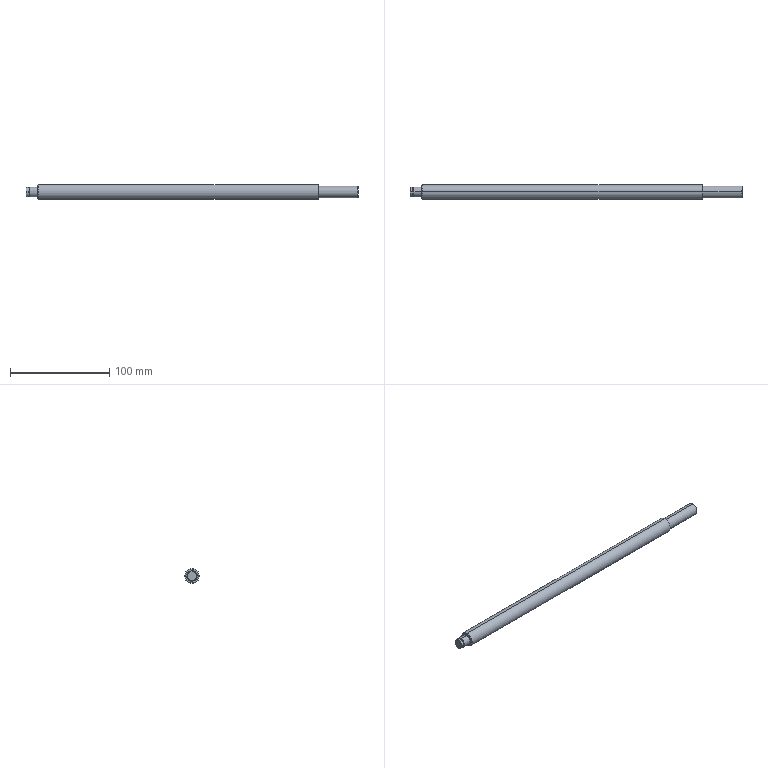Part | SolidWorks | features BaseBody 1 | 1 solid | 26 faces | box 335 x 15 x 15 mm | volume 55455 mm3 | cylinder 10 | cone 6 | plane 6 | spline 4 | commonest cylinder face diameters 10 x4 9.6 x2 12 x2 15 x2
STEP:
#1=CARTESIAN_POINT('',(295.3,0.,-6.));
#2=VERTEX_POINT('',#1);
#3=CARTESIAN_POINT('',(295.3,0.,6.));
#4=VERTEX_POINT('',#3);
#5=CARTESIAN_POINT('',(295.3,0.,0.));
#6=DIRECTION('',(1.,0.,0.));
#7=DIRECTION('',(0.,0.,1.));
#8=AXIS2_PLACEMENT_3D('',#5,#6,#7);
#9=CIRCLE('',#8,6.);
#10=EDGE_CURVE('',#2,#4,#9,.T.);
#11=ORIENTED_EDGE('',*,*,#10,.F.);
#12=CARTESIAN_POINT('',(295.,0.,-6.3));
#13=VERTEX_POINT('',#12);
#14=CARTESIAN_POINT('',(295.3,0.,-6.3));
#15=DIRECTION('',(0.,-1.,0.));
#16=DIRECTION('',(0.,0.,-1.));
#17=AXIS2_PLACEMENT_3D('',#14,#15,#16);
#18=CIRCLE('',#17,0.3);
#19=EDGE_CURVE('',#2,#13,#18,.T.);
#20=ORIENTED_EDGE('',*,*,#19,.T.);
#21=CARTESIAN_POINT('',(295.,0.,6.3));
#22=VERTEX_POINT('',#21);
#23=CARTESIAN_POINT('',(295.,0.,-6.3));
#24=CARTESIAN_POINT('',(295.,12.6,-6.3));
#25=CARTESIAN_POINT('',(295.,12.6,6.3));
#26=CARTESIAN_POINT('',(295.,0.,6.3));
#27=(BOUNDED_CURVE()B_SPLINE_CURVE(3,(#23,#24,#25,#26),.UNSPECIFIED.,.F.,.F.)B_SPLINE_CURVE_WITH_KNOTS((4,4),(0.,1.),.UNSPECIFIED.)CURVE()GEOMETRIC_REPRESENTATION_ITEM()RATIONAL_B_SPLINE_CURVE((1.,0.3333,0.3333,1.))REPRESENTATION_ITEM(''));
#28=EDGE_CURVE('',#13,#22,#27,.T.);
#29=ORIENTED_EDGE('',*,*,#28,.T.);
#30=CARTESIAN_POINT('',(295.3,0.,6.3));
#31=DIRECTION('',(0.,1.,0.));
#32=DIRECTION('',(0.,0.,1.));
#33=AXIS2_PLACEMENT_3D('',#30,#31,#32);
#34=CIRCLE('',#33,0.3);
#35=EDGE_CURVE('',#4,#22,#34,.T.);
#36=ORIENTED_EDGE('',*,*,#35,.F.);
#37=EDGE_LOOP('',(#11,#20,#29,#36));
#38=FACE_OUTER_BOUND('',#37,.T.);
#39=CARTESIAN_POINT('',(295.3,0.,6.));
#40=CARTESIAN_POINT('',(295.3,12.,6.));
#41=CARTESIAN_POINT('',(295.3,12.,-6.));
#42=CARTESIAN_POINT('',(295.3,0.,-6.));
#43=CARTESIAN_POINT('',(295.124,0.,6.));
#44=CARTESIAN_POINT('',(295.124,12.,6.));
#45=CARTESIAN_POINT('',(295.124,12.,-6.));
#46=CARTESIAN_POINT('',(295.124,0.,-6.));
#47=CARTESIAN_POINT('',(295.,0.,6.124));
#48=CARTESIAN_POINT('',(295.,12.249,6.124));
#49=CARTESIAN_POINT('',(295.,12.249,-6.124));
#50=CARTESIAN_POINT('',(295.,0.,-6.124));
#51=CARTESIAN_POINT('',(295.,0.,6.3));
#52=CARTESIAN_POINT('',(295.,12.6,6.3));
#53=CARTESIAN_POINT('',(295.,12.6,-6.3));
#54=CARTESIAN_POINT('',(295.,0.,-6.3));
#55=(BOUNDED_SURFACE()B_SPLINE_SURFACE(3,3,((#39,#40,#41,#42),(#43,#44,#45,#46),(#47,#48,#49,#50),(#51,#52,#53,#54)),.UNSPECIFIED.,.F.,.F.,.T.)B_SPLINE_SURFACE_WITH_KNOTS((4,4),(4,4),(0.,1.),(0.,1.),.UNSPECIFIED.)GEOMETRIC_REPRESENTATION_ITEM()RATIONAL_B_SPLINE_SURFACE(((1.,0.3333,0.3333,1.),(0.8047,0.2682,0.2682,0.8047),(0.8047,0.2682,0.2682,0.8047),(1.,0.3333,0.3333,1.)))REPRESENTATION_ITEM('')SURFACE());
#56=ADVANCED_FACE('',(#38),#55,.F.);
#57=CARTESIAN_POINT('',(12.,0.,5.3));
#58=VERTEX_POINT('',#57);
#59=CARTESIAN_POINT('',(12.,0.,-5.3));
#60=VERTEX_POINT('',#59);
#61=CARTESIAN_POINT('',(12.,0.,5.3));
#62=CARTESIAN_POINT('',(12.,10.6,5.3));
#63=CARTESIAN_POINT('',(12.,10.6,-5.3));
#64=CARTESIAN_POINT('',(12.,0.,-5.3));
#65=(BOUNDED_CURVE()B_SPLINE_CURVE(3,(#61,#62,#63,#64),.UNSPECIFIED.,.F.,.F.)B_SPLINE_CURVE_WITH_KNOTS((4,4),(0.,1.),.UNSPECIFIED.)CURVE()GEOMETRIC_REPRESENTATION_ITEM()RATIONAL_B_SPLINE_CURVE((1.,0.3333,0.3333,1.))REPRESENTATION_ITEM(''));
#66=EDGE_CURVE('',#58,#60,#65,.T.);
#67=ORIENTED_EDGE('',*,*,#66,.T.);
#68=CARTESIAN_POINT('',(11.7,0.,-5.));
#69=VERTEX_POINT('',#68);
#70=CARTESIAN_POINT('',(11.7,0.,-5.3));
#71=DIRECTION('',(0.,-1.,0.));
#72=DIRECTION('',(0.,0.,-1.));
#73=AXIS2_PLACEMENT_3D('',#70,#71,#72);
#74=CIRCLE('',#73,0.3);
#75=EDGE_CURVE('',#60,#69,#74,.T.);
#76=ORIENTED_EDGE('',*,*,#75,.T.);
#77=CARTESIAN_POINT('',(11.7,0.,5.));
#78=VERTEX_POINT('',#77);
#79=CARTESIAN_POINT('',(11.7,0.,0.));
#80=DIRECTION('',(-1.,0.,0.));
#81=DIRECTION('',(0.,0.,1.));
#82=AXIS2_PLACEMENT_3D('',#79,#80,#81);
#83=CIRCLE('',#82,5.);
#84=EDGE_CURVE('',#78,#69,#83,.T.);
#85=ORIENTED_EDGE('',*,*,#84,.F.);
#86=CARTESIAN_POINT('',(11.7,0.,5.3));
#87=DIRECTION('',(0.,1.,0.));
#88=DIRECTION('',(0.,0.,1.));
#89=AXIS2_PLACEMENT_3D('',#86,#87,#88);
#90=CIRCLE('',#89,0.3);
#91=EDGE_CURVE('',#58,#78,#90,.T.);
#92=ORIENTED_EDGE('',*,*,#91,.F.);
#93=EDGE_LOOP('',(#67,#76,#85,#92));
#94=FACE_OUTER_BOUND('',#93,.T.);
#95=CARTESIAN_POINT('',(12.,0.,5.3));
#96=CARTESIAN_POINT('',(12.,10.6,5.3));
#97=CARTESIAN_POINT('',(12.,10.6,-5.3));
#98=CARTESIAN_POINT('',(12.,0.,-5.3));
#99=CARTESIAN_POINT('',(12.,0.,5.124));
#100=CARTESIAN_POINT('',(12.,10.249,5.124));
#101=CARTESIAN_POINT('',(12.,10.249,-5.124));
#102=CARTESIAN_POINT('',(12.,0.,-5.124));
#103=CARTESIAN_POINT('',(11.876,0.,5.));
#104=CARTESIAN_POINT('',(11.876,10.,5.));
#105=CARTESIAN_POINT('',(11.876,10.,-5.));
#106=CARTESIAN_POINT('',(11.876,0.,-5.));
#107=CARTESIAN_POINT('',(11.7,0.,5.));
#108=CARTESIAN_POINT('',(11.7,10.,5.));
#109=CARTESIAN_POINT('',(11.7,10.,-5.));
#110=CARTESIAN_POINT('',(11.7,0.,-5.));
#111=(BOUNDED_SURFACE()B_SPLINE_SURFACE(3,3,((#95,#96,#97,#98),(#99,#100,#101,#102),(#103,#104,#105,#106),(#107,#108,#109,#110)),.UNSPECIFIED.,.F.,.F.,.T.)B_SPLINE_SURFACE_WITH_KNOTS((4,4),(4,4),(0.,1.),(0.,1.),.UNSPECIFIED.)GEOMETRIC_REPRESENTATION_ITEM()RATIONAL_B_SPLINE_SURFACE(((1.,0.3333,0.3333,1.),(0.8047,0.2682,0.2682,0.8047),(0.8047,0.2682,0.2682,0.8047),(1.,0.3333,0.3333,1.)))REPRESENTATION_ITEM('')SURFACE());
#112=ADVANCED_FACE('',(#94),#111,.F.);
#113=CARTESIAN_POINT('',(295.,0.,7.5));
#114=VERTEX_POINT('',#113);
#115=CARTESIAN_POINT('',(295.,0.,-7.5));
#116=VERTEX_POINT('',#115);
#117=CARTESIAN_POINT('',(295.,0.,0.));
#118=DIRECTION('',(-1.,0.,0.));
#119=DIRECTION('',(0.,0.,1.));
#120=AXIS2_PLACEMENT_3D('',#117,#118,#119);
#121=CIRCLE('',#120,7.5);
#122=EDGE_CURVE('',#114,#116,#121,.T.);
#123=ORIENTED_EDGE('',*,*,#122,.T.);
#124=CARTESIAN_POINT('',(12.5,0.,-7.5));
#125=VERTEX_POINT('',#124);
#126=CARTESIAN_POINT('',(350.,0.,-7.5));
#127=DIRECTION('',(-1.,0.,0.));
#128=VECTOR('',#127,1000.);
#129=LINE('',#126,#128);
#130=EDGE_CURVE('',#116,#125,#129,.T.);
#131=ORIENTED_EDGE('',*,*,#130,.T.);
#132=CARTESIAN_POINT('',(12.5,0.,7.5));
#133=VERTEX_POINT('',#132);
#134=CARTESIAN_POINT('',(12.5,0.,0.));
#135=DIRECTION('',(1.,0.,0.));
#136=DIRECTION('',(0.,0.,1.));
#137=AXIS2_PLACEMENT_3D('',#134,#135,#136);
#138=CIRCLE('',#137,7.5);
#139=EDGE_CURVE('',#125,#133,#138,.T.);
#140=ORIENTED_EDGE('',*,*,#139,.T.);
#141=CARTESIAN_POINT('',(350.,0.,7.5));
#142=DIRECTION('',(-1.,0.,0.));
#143=VECTOR('',#142,1000.);
#144=LINE('',#141,#143);
#145=EDGE_CURVE('',#114,#133,#144,.T.);
#146=ORIENTED_EDGE('',*,*,#145,.F.);
#147=EDGE_LOOP('',(#123,#131,#140,#146));
#148=FACE_OUTER_BOUND('',#147,.T.);
#149=CARTESIAN_POINT('',(350.,0.,0.));
#150=DIRECTION('',(-1.,0.,0.));
#151=DIRECTION('',(0.,0.,1.));
#152=AXIS2_PLACEMENT_3D('',#149,#150,#151);
#153=CYLINDRICAL_SURFACE('',#152,7.5);
#154=ADVANCED_FACE('',(#148),#153,.T.);
#155=CARTESIAN_POINT('',(12.,0.,-7.));
#156=VERTEX_POINT('',#155);
#157=CARTESIAN_POINT('',(12.,0.,7.));
#158=VERTEX_POINT('',#157);
#159=CARTESIAN_POINT('',(12.,0.,0.));
#160=DIRECTION('',(1.,0.,0.));
#161=DIRECTION('',(0.,0.,-1.));
#162=AXIS2_PLACEMENT_3D('',#159,#160,#161);
#163=CIRCLE('',#162,7.);
#164=EDGE_CURVE('',#156,#158,#163,.T.);
#165=ORIENTED_EDGE('',*,*,#164,.T.);
#166=CARTESIAN_POINT('',(12.5,0.,7.5));
#167=DIRECTION('',(0.7071,0.,0.7071));
#168=VECTOR('',#167,1000.);
#169=LINE('',#166,#168);
#170=EDGE_CURVE('',#158,#133,#169,.T.);
#171=ORIENTED_EDGE('',*,*,#170,.T.);
#172=ORIENTED_EDGE('',*,*,#139,.F.);
#173=CARTESIAN_POINT('',(12.5,0.,-7.5));
#174=DIRECTION('',(0.7071,0.,-0.7071));
#175=VECTOR('',#174,1000.);
#176=LINE('',#173,#175);
#177=EDGE_CURVE('',#156,#125,#176,.T.);
#178=ORIENTED_EDGE('',*,*,#177,.F.);
#179=EDGE_LOOP('',(#165,#171,#172,#178));
#180=FACE_OUTER_BOUND('',#179,.T.);
#181=CARTESIAN_POINT('',(12.5,0.,0.));
#182=DIRECTION('',(1.,0.,0.));
#183=DIRECTION('',(0.,0.,-1.));
#184=AXIS2_PLACEMENT_3D('',#181,#182,#183);
#185=CONICAL_SURFACE('',#184,7.5,0.7854);
#186=ADVANCED_FACE('',(#180),#185,.T.);
#187=CARTESIAN_POINT('',(334.5,0.,6.));
#188=VERTEX_POINT('',#187);
#189=CARTESIAN_POINT('',(334.5,0.,-6.));
#190=VERTEX_POINT('',#189);
#191=CARTESIAN_POINT('',(334.5,0.,0.));
#192=DIRECTION('',(-1.,0.,0.));
#193=DIRECTION('',(0.,0.,1.));
#194=AXIS2_PLACEMENT_3D('',#191,#192,#193);
#195=CIRCLE('',#194,6.);
#196=EDGE_CURVE('',#188,#190,#195,.T.);
#197=ORIENTED_EDGE('',*,*,#196,.T.);
#198=CARTESIAN_POINT('',(350.,0.,-6.));
#199=DIRECTION('',(-1.,0.,0.));
#200=VECTOR('',#199,1000.);
#201=LINE('',#198,#200);
#202=EDGE_CURVE('',#190,#2,#201,.T.);
#203=ORIENTED_EDGE('',*,*,#202,.T.);
#204=ORIENTED_EDGE('',*,*,#10,.T.);
#205=CARTESIAN_POINT('',(350.,0.,6.));
#206=DIRECTION('',(-1.,0.,0.));
#207=VECTOR('',#206,1000.);
#208=LINE('',#205,#207);
#209=EDGE_CURVE('',#188,#4,#208,.T.);
#210=ORIENTED_EDGE('',*,*,#209,.F.);
#211=EDGE_LOOP('',(#197,#203,#204,#210));
#212=FACE_OUTER_BOUND('',#211,.T.);
#213=CARTESIAN_POINT('',(350.,0.,0.));
#214=DIRECTION('',(-1.,0.,0.));
#215=DIRECTION('',(0.,0.,1.));
#216=AXIS2_PLACEMENT_3D('',#213,#214,#215);
#217=CYLINDRICAL_SURFACE('',#216,6.);
#218=ADVANCED_FACE('',(#212),#217,.T.);
#219=ORIENTED_EDGE('',*,*,#84,.T.);
#220=CARTESIAN_POINT('',(4.,0.,-5.));
#221=VERTEX_POINT('',#220);
#222=CARTESIAN_POINT('',(350.,0.,-5.));
#223=DIRECTION('',(-1.,0.,0.));
#224=VECTOR('',#223,1000.);
#225=LINE('',#222,#224);
#226=EDGE_CURVE('',#69,#221,#225,.T.);
#227=ORIENTED_EDGE('',*,*,#226,.T.);
#228=CARTESIAN_POINT('',(4.,0.,5.));
#229=VERTEX_POINT('',#228);
#230=CARTESIAN_POINT('',(4.,0.,0.));
#231=DIRECTION('',(1.,0.,0.));
#232=DIRECTION('',(0.,0.,1.));
#233=AXIS2_PLACEMENT_3D('',#230,#231,#232);
#234=CIRCLE('',#233,5.);
#235=EDGE_CURVE('',#221,#229,#234,.T.);
#236=ORIENTED_EDGE('',*,*,#235,.T.);
#237=CARTESIAN_POINT('',(350.,0.,5.));
#238=DIRECTION('',(-1.,0.,0.));
#239=VECTOR('',#238,1000.);
#240=LINE('',#237,#239);
#241=EDGE_CURVE('',#78,#229,#240,.T.);
#242=ORIENTED_EDGE('',*,*,#241,.F.);
#243=EDGE_LOOP('',(#219,#227,#236,#242));
#244=FACE_OUTER_BOUND('',#243,.T.);
#245=CARTESIAN_POINT('',(350.,0.,0.));
#246=DIRECTION('',(-1.,0.,0.));
#247=DIRECTION('',(0.,0.,1.));
#248=AXIS2_PLACEMENT_3D('',#245,#246,#247);
#249=CYLINDRICAL_SURFACE('',#248,5.);
#250=ADVANCED_FACE('',(#244),#249,.T.);
#251=CARTESIAN_POINT('',(335.,0.,5.5));
#252=VERTEX_POINT('',#251);
#253=CARTESIAN_POINT('',(335.,0.,-5.5));
#254=VERTEX_POINT('',#253);
#255=CARTESIAN_POINT('',(335.,0.,0.));
#256=DIRECTION('',(-1.,0.,0.));
#257=DIRECTION('',(0.,0.,1.));
#258=AXIS2_PLACEMENT_3D('',#255,#256,#257);
#259=CIRCLE('',#258,5.5);
#260=EDGE_CURVE('',#252,#254,#259,.T.);
#261=ORIENTED_EDGE('',*,*,#260,.T.);
#262=CARTESIAN_POINT('',(334.5,0.,-6.));
#263=DIRECTION('',(-0.7071,0.,-0.7071));
#264=VECTOR('',#263,1000.);
#265=LINE('',#262,#264);
#266=EDGE_CURVE('',#254,#190,#265,.T.);
#267=ORIENTED_EDGE('',*,*,#266,.T.);
#268=ORIENTED_EDGE('',*,*,#196,.F.);
#269=CARTESIAN_POINT('',(334.5,0.,6.));
#270=DIRECTION('',(-0.7071,0.,0.7071));
#271=VECTOR('',#270,1000.);
#272=LINE('',#269,#271);
#273=EDGE_CURVE('',#252,#188,#272,.T.);
#274=ORIENTED_EDGE('',*,*,#273,.F.);
#275=EDGE_LOOP('',(#261,#267,#268,#274));
#276=FACE_OUTER_BOUND('',#275,.T.);
#277=CARTESIAN_POINT('',(334.5,0.,0.));
#278=DIRECTION('',(-1.,0.,0.));
#279=DIRECTION('',(0.,0.,1.));
#280=AXIS2_PLACEMENT_3D('',#277,#278,#279);
#281=CONICAL_SURFACE('',#280,6.,0.7854);
#282=ADVANCED_FACE('',(#276),#281,.T.);
#283=CARTESIAN_POINT('',(4.,0.,4.8));
#284=VERTEX_POINT('',#283);
#285=CARTESIAN_POINT('',(4.,0.,-4.8));
#286=VERTEX_POINT('',#285);
#287=CARTESIAN_POINT('',(4.,0.,0.));
#288=DIRECTION('',(-1.,0.,0.));
#289=DIRECTION('',(0.,0.,1.));
#290=AXIS2_PLACEMENT_3D('',#287,#288,#289);
#291=CIRCLE('',#290,4.8);
#292=EDGE_CURVE('',#284,#286,#291,.T.);
#293=ORIENTED_EDGE('',*,*,#292,.T.);
#294=CARTESIAN_POINT('',(2.85,0.,-4.8));
#295=VERTEX_POINT('',#294);
#296=CARTESIAN_POINT('',(350.,0.,-4.8));
#297=DIRECTION('',(-1.,0.,0.));
#298=VECTOR('',#297,1000.);
#299=LINE('',#296,#298);
#300=EDGE_CURVE('',#286,#295,#299,.T.);
#301=ORIENTED_EDGE('',*,*,#300,.T.);
#302=CARTESIAN_POINT('',(2.85,0.,4.8));
#303=VERTEX_POINT('',#302);
#304=CARTESIAN_POINT('',(2.85,0.,0.));
#305=DIRECTION('',(1.,0.,0.));
#306=DIRECTION('',(0.,0.,1.));
#307=AXIS2_PLACEMENT_3D('',#304,#305,#306);
#308=CIRCLE('',#307,4.8);
#309=EDGE_CURVE('',#295,#303,#308,.T.);
#310=ORIENTED_EDGE('',*,*,#309,.T.);
#311=CARTESIAN_POINT('',(350.,0.,4.8));
#312=DIRECTION('',(-1.,0.,0.));
#313=VECTOR('',#312,1000.);
#314=LINE('',#311,#313);
#315=EDGE_CURVE('',#284,#303,#314,.T.);
#316=ORIENTED_EDGE('',*,*,#315,.F.);
#317=EDGE_LOOP('',(#293,#301,#310,#316));
#318=FACE_OUTER_BOUND('',#317,.T.);
#319=CARTESIAN_POINT('',(350.,0.,0.));
#320=DIRECTION('',(-1.,0.,0.));
#321=DIRECTION('',(0.,0.,1.));
#322=AXIS2_PLACEMENT_3D('',#319,#320,#321);
#323=CYLINDRICAL_SURFACE('',#322,4.8);
#324=ADVANCED_FACE('',(#318),#323,.T.);
#325=CARTESIAN_POINT('',(2.85,0.,5.));
#326=VERTEX_POINT('',#325);
#327=CARTESIAN_POINT('',(2.85,0.,-5.));
#328=VERTEX_POINT('',#327);
#329=CARTESIAN_POINT('',(2.85,0.,0.));
#330=DIRECTION('',(-1.,0.,0.));
#331=DIRECTION('',(0.,0.,1.));
#332=AXIS2_PLACEMENT_3D('',#329,#330,#331);
#333=CIRCLE('',#332,5.);
#334=EDGE_CURVE('',#326,#328,#333,.T.);
#335=ORIENTED_EDGE('',*,*,#334,.T.);
#336=CARTESIAN_POINT('',(0.5,0.,-5.));
#337=VERTEX_POINT('',#336);
#338=CARTESIAN_POINT('',(350.,0.,-5.));
#339=DIRECTION('',(-1.,0.,0.));
#340=VECTOR('',#339,1000.);
#341=LINE('',#338,#340);
#342=EDGE_CURVE('',#328,#337,#341,.T.);
#343=ORIENTED_EDGE('',*,*,#342,.T.);
#344=CARTESIAN_POINT('',(0.5,0.,5.));
#345=VERTEX_POINT('',#344);
#346=CARTESIAN_POINT('',(0.5,0.,0.));
#347=DIRECTION('',(1.,0.,0.));
#348=DIRECTION('',(0.,0.,1.));
#349=AXIS2_PLACEMENT_3D('',#346,#347,#348);
#350=CIRCLE('',#349,5.);
#351=EDGE_CURVE('',#337,#345,#350,.T.);
#352=ORIENTED_EDGE('',*,*,#351,.T.);
#353=CARTESIAN_POINT('',(350.,0.,5.));
#354=DIRECTION('',(-1.,0.,0.));
#355=VECTOR('',#354,1000.);
#356=LINE('',#353,#355);
#357=EDGE_CURVE('',#326,#345,#356,.T.);
#358=ORIENTED_EDGE('',*,*,#357,.F.);
#359=EDGE_LOOP('',(#335,#343,#352,#358));
#360=FACE_OUTER_BOUND('',#359,.T.);
#361=CARTESIAN_POINT('',(350.,0.,0.));
#362=DIRECTION('',(-1.,0.,0.));
#363=DIRECTION('',(0.,0.,1.));
#364=AXIS2_PLACEMENT_3D('',#361,#362,#363);
#365=CYLINDRICAL_SURFACE('',#364,5.);
#366=ADVANCED_FACE('',(#360),#365,.T.);
#367=CARTESIAN_POINT('',(0.,0.,-4.5));
#368=VERTEX_POINT('',#367);
#369=CARTESIAN_POINT('',(0.,0.,4.5));
#370=VERTEX_POINT('',#369);
#371=CARTESIAN_POINT('',(0.,0.,0.));
#372=DIRECTION('',(1.,0.,0.));
#373=DIRECTION('',(0.,0.,-1.));
#374=AXIS2_PLACEMENT_3D('',#371,#372,#373);
#375=CIRCLE('',#374,4.5);
#376=EDGE_CURVE('',#368,#370,#375,.T.);
#377=ORIENTED_EDGE('',*,*,#376,.T.);
#378=CARTESIAN_POINT('',(0.5,0.,5.));
#379=DIRECTION('',(0.7071,0.,0.7071));
#380=VECTOR('',#379,1000.);
#381=LINE('',#378,#380);
#382=EDGE_CURVE('',#370,#345,#381,.T.);
#383=ORIENTED_EDGE('',*,*,#382,.T.);
#384=ORIENTED_EDGE('',*,*,#351,.F.);
#385=CARTESIAN_POINT('',(0.5,0.,-5.));
#386=DIRECTION('',(0.7071,0.,-0.7071));
#387=VECTOR('',#386,1000.);
#388=LINE('',#385,#387);
#389=EDGE_CURVE('',#368,#337,#388,.T.);
#390=ORIENTED_EDGE('',*,*,#389,.F.);
#391=EDGE_LOOP('',(#377,#383,#384,#390));
#392=FACE_OUTER_BOUND('',#391,.T.);
#393=CARTESIAN_POINT('',(0.5,0.,0.));
#394=DIRECTION('',(1.,0.,0.));
#395=DIRECTION('',(0.,0.,-1.));
#396=AXIS2_PLACEMENT_3D('',#393,#394,#395);
#397=CONICAL_SURFACE('',#396,5.,0.7854);
#398=ADVANCED_FACE('',(#392),#397,.T.);
#399=ORIENTED_EDGE('',*,*,#130,.F.);
#400=CARTESIAN_POINT('',(295.,0.,0.));
#401=DIRECTION('',(-1.,0.,0.));
#402=DIRECTION('',(0.,0.,1.));
#403=AXIS2_PLACEMENT_3D('',#400,#401,#402);
#404=CIRCLE('',#403,7.5);
#405=EDGE_CURVE('',#116,#114,#404,.T.);
#406=ORIENTED_EDGE('',*,*,#405,.T.);
#407=ORIENTED_EDGE('',*,*,#145,.T.);
#408=CARTESIAN_POINT('',(12.5,0.,0.));
#409=DIRECTION('',(1.,0.,0.));
#410=DIRECTION('',(0.,0.,1.));
#411=AXIS2_PLACEMENT_3D('',#408,#409,#410);
#412=CIRCLE('',#411,7.5);
#413=EDGE_CURVE('',#133,#125,#412,.T.);
#414=ORIENTED_EDGE('',*,*,#413,.T.);
#415=EDGE_LOOP('',(#399,#406,#407,#414));
#416=FACE_OUTER_BOUND('',#415,.T.);
#417=CARTESIAN_POINT('',(350.,0.,0.));
#418=DIRECTION('',(-1.,0.,0.));
#419=DIRECTION('',(0.,0.,1.));
#420=AXIS2_PLACEMENT_3D('',#417,#418,#419);
#421=CYLINDRICAL_SURFACE('',#420,7.5);
#422=ADVANCED_FACE('',(#416),#421,.T.);
#423=ORIENTED_EDGE('',*,*,#170,.F.);
#424=CARTESIAN_POINT('',(12.,0.,0.));
#425=DIRECTION('',(1.,0.,0.));
#426=DIRECTION('',(0.,0.,-1.));
#427=AXIS2_PLACEMENT_3D('',#424,#425,#426);
#428=CIRCLE('',#427,7.);
#429=EDGE_CURVE('',#158,#156,#428,.T.);
#430=ORIENTED_EDGE('',*,*,#429,.T.);
#431=ORIENTED_EDGE('',*,*,#177,.T.);
#432=ORIENTED_EDGE('',*,*,#413,.F.);
#433=EDGE_LOOP('',(#423,#430,#431,#432));
#434=FACE_OUTER_BOUND('',#433,.T.);
#435=CARTESIAN_POINT('',(12.5,0.,0.));
#436=DIRECTION('',(1.,0.,0.));
#437=DIRECTION('',(0.,0.,-1.));
#438=AXIS2_PLACEMENT_3D('',#435,#436,#437);
#439=CONICAL_SURFACE('',#438,7.5,0.7854);
#440=ADVANCED_FACE('',(#434),#439,.T.);
#441=CARTESIAN_POINT('',(295.,0.,6.3));
#442=CARTESIAN_POINT('',(295.,-12.6,6.3));
#443=CARTESIAN_POINT('',(295.,-12.6,-6.3));
#444=CARTESIAN_POINT('',(295.,0.,-6.3));
#445=(BOUNDED_CURVE()B_SPLINE_CURVE(3,(#441,#442,#443,#444),.UNSPECIFIED.,.F.,.F.)B_SPLINE_CURVE_WITH_KNOTS((4,4),(0.,1.),.UNSPECIFIED.)CURVE()GEOMETRIC_REPRESENTATION_ITEM()RATIONAL_B_SPLINE_CURVE((1.,0.3333,0.3333,1.))REPRESENTATION_ITEM(''));
#446=EDGE_CURVE('',#22,#13,#445,.T.);
#447=ORIENTED_EDGE('',*,*,#446,.F.);
#448=ORIENTED_EDGE('',*,*,#28,.F.);
#449=EDGE_LOOP('',(#447,#448));
#450=FACE_BOUND('',#449,.T.);
#451=ORIENTED_EDGE('',*,*,#122,.F.);
#452=ORIENTED_EDGE('',*,*,#405,.F.);
#453=EDGE_LOOP('',(#451,#452));
#454=FACE_OUTER_BOUND('',#453,.T.);
#455=CARTESIAN_POINT('',(295.,7.5,0.));
#456=DIRECTION('',(-1.,0.,0.));
#457=DIRECTION('',(0.,0.,1.));
#458=AXIS2_PLACEMENT_3D('',#455,#456,#457);
#459=PLANE('',#458);
#460=ADVANCED_FACE('',(#450,#454),#459,.F.);
#461=ORIENTED_EDGE('',*,*,#164,.F.);
#462=ORIENTED_EDGE('',*,*,#429,.F.);
#463=EDGE_LOOP('',(#461,#462));
#464=FACE_OUTER_BOUND('',#463,.T.);
#465=CARTESIAN_POINT('',(12.,0.,-5.3));
#466=CARTESIAN_POINT('',(12.,-10.6,-5.3));
#467=CARTESIAN_POINT('',(12.,-10.6,5.3));
#468=CARTESIAN_POINT('',(12.,0.,5.3));
#469=(BOUNDED_CURVE()B_SPLINE_CURVE(3,(#465,#466,#467,#468),.UNSPECIFIED.,.F.,.F.)B_SPLINE_CURVE_WITH_KNOTS((4,4),(0.,1.),.UNSPECIFIED.)CURVE()GEOMETRIC_REPRESENTATION_ITEM()RATIONAL_B_SPLINE_CURVE((1.,0.3333,0.3333,1.))REPRESENTATION_ITEM(''));
#470=EDGE_CURVE('',#60,#58,#469,.T.);
#471=ORIENTED_EDGE('',*,*,#470,.F.);
#472=ORIENTED_EDGE('',*,*,#66,.F.);
#473=EDGE_LOOP('',(#471,#472));
#474=FACE_BOUND('',#473,.T.);
#475=CARTESIAN_POINT('',(12.,5.3,0.));
#476=DIRECTION('',(1.,0.,0.));
#477=DIRECTION('',(0.,0.,-1.));
#478=AXIS2_PLACEMENT_3D('',#475,#476,#477);
#479=PLANE('',#478);
#480=ADVANCED_FACE('',(#464,#474),#479,.F.);
#481=ORIENTED_EDGE('',*,*,#19,.F.);
#482=CARTESIAN_POINT('',(295.3,0.,0.));
#483=DIRECTION('',(1.,0.,0.));
#484=DIRECTION('',(0.,0.,1.));
#485=AXIS2_PLACEMENT_3D('',#482,#483,#484);
#486=CIRCLE('',#485,6.);
#487=EDGE_CURVE('',#4,#2,#486,.T.);
#488=ORIENTED_EDGE('',*,*,#487,.F.);
#489=ORIENTED_EDGE('',*,*,#35,.T.);
#490=ORIENTED_EDGE('',*,*,#446,.T.);
#491=EDGE_LOOP('',(#481,#488,#489,#490));
#492=FACE_OUTER_BOUND('',#491,.T.);
#493=CARTESIAN_POINT('',(295.3,0.,-6.));
#494=CARTESIAN_POINT('',(295.3,-12.,-6.));
#495=CARTESIAN_POINT('',(295.3,-12.,6.));
#496=CARTESIAN_POINT('',(295.3,0.,6.));
#497=CARTESIAN_POINT('',(295.124,0.,-6.));
#498=CARTESIAN_POINT('',(295.124,-12.,-6.));
#499=CARTESIAN_POINT('',(295.124,-12.,6.));
#500=CARTESIAN_POINT('',(295.124,0.,6.));
#501=CARTESIAN_POINT('',(295.,0.,-6.124));
#502=CARTESIAN_POINT('',(295.,-12.249,-6.124));
#503=CARTESIAN_POINT('',(295.,-12.249,6.124));
#504=CARTESIAN_POINT('',(295.,0.,6.124));
#505=CARTESIAN_POINT('',(295.,0.,-6.3));
#506=CARTESIAN_POINT('',(295.,-12.6,-6.3));
#507=CARTESIAN_POINT('',(295.,-12.6,6.3));
#508=CARTESIAN_POINT('',(295.,0.,6.3));
#509=(BOUNDED_SURFACE()B_SPLINE_SURFACE(3,3,((#493,#494,#495,#496),(#497,#498,#499,#500),(#501,#502,#503,#504),(#505,#506,#507,#508)),.UNSPECIFIED.,.F.,.F.,.T.)B_SPLINE_SURFACE_WITH_KNOTS((4,4),(4,4),(0.,1.),(0.,1.),.UNSPECIFIED.)GEOMETRIC_REPRESENTATION_ITEM()RATIONAL_B_SPLINE_SURFACE(((1.,0.3333,0.3333,1.),(0.8047,0.2682,0.2682,0.8047),(0.8047,0.2682,0.2682,0.8047),(1.,0.3333,0.3333,1.)))REPRESENTATION_ITEM('')SURFACE());
#510=ADVANCED_FACE('',(#492),#509,.F.);
#511=ORIENTED_EDGE('',*,*,#75,.F.);
#512=ORIENTED_EDGE('',*,*,#470,.T.);
#513=ORIENTED_EDGE('',*,*,#91,.T.);
#514=CARTESIAN_POINT('',(11.7,0.,0.));
#515=DIRECTION('',(-1.,0.,0.));
#516=DIRECTION('',(0.,0.,1.));
#517=AXIS2_PLACEMENT_3D('',#514,#515,#516);
#518=CIRCLE('',#517,5.);
#519=EDGE_CURVE('',#69,#78,#518,.T.);
#520=ORIENTED_EDGE('',*,*,#519,.F.);
#521=EDGE_LOOP('',(#511,#512,#513,#520));
#522=FACE_OUTER_BOUND('',#521,.T.);
#523=CARTESIAN_POINT('',(12.,0.,-5.3));
#524=CARTESIAN_POINT('',(12.,-10.6,-5.3));
#525=CARTESIAN_POINT('',(12.,-10.6,5.3));
#526=CARTESIAN_POINT('',(12.,0.,5.3));
#527=CARTESIAN_POINT('',(12.,0.,-5.124));
#528=CARTESIAN_POINT('',(12.,-10.249,-5.124));
#529=CARTESIAN_POINT('',(12.,-10.249,5.124));
#530=CARTESIAN_POINT('',(12.,0.,5.124));
#531=CARTESIAN_POINT('',(11.876,0.,-5.));
#532=CARTESIAN_POINT('',(11.876,-10.,-5.));
#533=CARTESIAN_POINT('',(11.876,-10.,5.));
#534=CARTESIAN_POINT('',(11.876,0.,5.));
#535=CARTESIAN_POINT('',(11.7,0.,-5.));
#536=CARTESIAN_POINT('',(11.7,-10.,-5.));
#537=CARTESIAN_POINT('',(11.7,-10.,5.));
#538=CARTESIAN_POINT('',(11.7,0.,5.));
#539=(BOUNDED_SURFACE()B_SPLINE_SURFACE(3,3,((#523,#524,#525,#526),(#527,#528,#529,#530),(#531,#532,#533,#534),(#535,#536,#537,#538)),.UNSPECIFIED.,.F.,.F.,.F.)B_SPLINE_SURFACE_WITH_KNOTS((4,4),(4,4),(0.,1.),(0.,1.),.UNSPECIFIED.)GEOMETRIC_REPRESENTATION_ITEM()RATIONAL_B_SPLINE_SURFACE(((1.,0.3333,0.3333,1.),(0.8047,0.2682,0.2682,0.8047),(0.8047,0.2682,0.2682,0.8047),(1.,0.3333,0.3333,1.)))REPRESENTATION_ITEM('')SURFACE());
#540=ADVANCED_FACE('',(#522),#539,.F.);
#541=ORIENTED_EDGE('',*,*,#202,.F.);
#542=CARTESIAN_POINT('',(334.5,0.,0.));
#543=DIRECTION('',(-1.,0.,0.));
#544=DIRECTION('',(0.,0.,1.));
#545=AXIS2_PLACEMENT_3D('',#542,#543,#544);
#546=CIRCLE('',#545,6.);
#547=EDGE_CURVE('',#190,#188,#546,.T.);
#548=ORIENTED_EDGE('',*,*,#547,.T.);
#549=ORIENTED_EDGE('',*,*,#209,.T.);
#550=ORIENTED_EDGE('',*,*,#487,.T.);
#551=EDGE_LOOP('',(#541,#548,#549,#550));
#552=FACE_OUTER_BOUND('',#551,.T.);
#553=CARTESIAN_POINT('',(350.,0.,0.));
#554=DIRECTION('',(-1.,0.,0.));
#555=DIRECTION('',(0.,0.,1.));
#556=AXIS2_PLACEMENT_3D('',#553,#554,#555);
#557=CYLINDRICAL_SURFACE('',#556,6.);
#558=ADVANCED_FACE('',(#552),#557,.T.);
#559=ORIENTED_EDGE('',*,*,#226,.F.);
#560=ORIENTED_EDGE('',*,*,#519,.T.);
#561=ORIENTED_EDGE('',*,*,#241,.T.);
#562=CARTESIAN_POINT('',(4.,0.,0.));
#563=DIRECTION('',(1.,0.,0.));
#564=DIRECTION('',(0.,0.,1.));
#565=AXIS2_PLACEMENT_3D('',#562,#563,#564);
#566=CIRCLE('',#565,5.);
#567=EDGE_CURVE('',#229,#221,#566,.T.);
#568=ORIENTED_EDGE('',*,*,#567,.T.);
#569=EDGE_LOOP('',(#559,#560,#561,#568));
#570=FACE_OUTER_BOUND('',#569,.T.);
#571=CARTESIAN_POINT('',(350.,0.,0.));
#572=DIRECTION('',(-1.,0.,0.));
#573=DIRECTION('',(0.,0.,1.));
#574=AXIS2_PLACEMENT_3D('',#571,#572,#573);
#575=CYLINDRICAL_SURFACE('',#574,5.);
#576=ADVANCED_FACE('',(#570),#575,.T.);
#577=ORIENTED_EDGE('',*,*,#266,.F.);
#578=CARTESIAN_POINT('',(335.,0.,0.));
#579=DIRECTION('',(-1.,0.,0.));
#580=DIRECTION('',(0.,0.,1.));
#581=AXIS2_PLACEMENT_3D('',#578,#579,#580);
#582=CIRCLE('',#581,5.5);
#583=EDGE_CURVE('',#254,#252,#582,.T.);
#584=ORIENTED_EDGE('',*,*,#583,.T.);
#585=ORIENTED_EDGE('',*,*,#273,.T.);
#586=ORIENTED_EDGE('',*,*,#547,.F.);
#587=EDGE_LOOP('',(#577,#584,#585,#586));
#588=FACE_OUTER_BOUND('',#587,.T.);
#589=CARTESIAN_POINT('',(334.5,0.,0.));
#590=DIRECTION('',(-1.,0.,0.));
#591=DIRECTION('',(0.,0.,1.));
#592=AXIS2_PLACEMENT_3D('',#589,#590,#591);
#593=CONICAL_SURFACE('',#592,6.,0.7854);
#594=ADVANCED_FACE('',(#588),#593,.T.);
#595=ORIENTED_EDGE('',*,*,#567,.F.);
#596=ORIENTED_EDGE('',*,*,#235,.F.);
#597=EDGE_LOOP('',(#595,#596));
#598=FACE_OUTER_BOUND('',#597,.T.);
#599=ORIENTED_EDGE('',*,*,#292,.F.);
#600=CARTESIAN_POINT('',(4.,0.,0.));
#601=DIRECTION('',(-1.,0.,0.));
#602=DIRECTION('',(0.,0.,1.));
#603=AXIS2_PLACEMENT_3D('',#600,#601,#602);
#604=CIRCLE('',#603,4.8);
#605=EDGE_CURVE('',#286,#284,#604,.T.);
#606=ORIENTED_EDGE('',*,*,#605,.F.);
#607=EDGE_LOOP('',(#599,#606));
#608=FACE_BOUND('',#607,.T.);
#609=CARTESIAN_POINT('',(4.,4.8,0.));
#610=DIRECTION('',(1.,0.,0.));
#611=DIRECTION('',(0.,0.,-1.));
#612=AXIS2_PLACEMENT_3D('',#609,#610,#611);
#613=PLANE('',#612);
#614=ADVANCED_FACE('',(#598,#608),#613,.F.);
#615=ORIENTED_EDGE('',*,*,#260,.F.);
#616=ORIENTED_EDGE('',*,*,#583,.F.);
#617=EDGE_LOOP('',(#615,#616));
#618=FACE_OUTER_BOUND('',#617,.T.);
#619=CARTESIAN_POINT('',(335.,5.5,0.));
#620=DIRECTION('',(-1.,0.,0.));
#621=DIRECTION('',(0.,0.,1.));
#622=AXIS2_PLACEMENT_3D('',#619,#620,#621);
#623=PLANE('',#622);
#624=ADVANCED_FACE('',(#618),#623,.F.);
#625=ORIENTED_EDGE('',*,*,#300,.F.);
#626=ORIENTED_EDGE('',*,*,#605,.T.);
#627=ORIENTED_EDGE('',*,*,#315,.T.);
#628=CARTESIAN_POINT('',(2.85,0.,0.));
#629=DIRECTION('',(1.,0.,0.));
#630=DIRECTION('',(0.,0.,1.));
#631=AXIS2_PLACEMENT_3D('',#628,#629,#630);
#632=CIRCLE('',#631,4.8);
#633=EDGE_CURVE('',#303,#295,#632,.T.);
#634=ORIENTED_EDGE('',*,*,#633,.T.);
#635=EDGE_LOOP('',(#625,#626,#627,#634));
#636=FACE_OUTER_BOUND('',#635,.T.);
#637=CARTESIAN_POINT('',(350.,0.,0.));
#638=DIRECTION('',(-1.,0.,0.));
#639=DIRECTION('',(0.,0.,1.));
#640=AXIS2_PLACEMENT_3D('',#637,#638,#639);
#641=CYLINDRICAL_SURFACE('',#640,4.8);
#642=ADVANCED_FACE('',(#636),#641,.T.);
#643=ORIENTED_EDGE('',*,*,#633,.F.);
#644=ORIENTED_EDGE('',*,*,#309,.F.);
#645=EDGE_LOOP('',(#643,#644));
#646=FACE_BOUND('',#645,.T.);
#647=ORIENTED_EDGE('',*,*,#334,.F.);
#648=CARTESIAN_POINT('',(2.85,0.,0.));
#649=DIRECTION('',(-1.,0.,0.));
#650=DIRECTION('',(0.,0.,1.));
#651=AXIS2_PLACEMENT_3D('',#648,#649,#650);
#652=CIRCLE('',#651,5.);
#653=EDGE_CURVE('',#328,#326,#652,.T.);
#654=ORIENTED_EDGE('',*,*,#653,.F.);
#655=EDGE_LOOP('',(#647,#654));
#656=FACE_OUTER_BOUND('',#655,.T.);
#657=CARTESIAN_POINT('',(2.85,5.,0.));
#658=DIRECTION('',(-1.,0.,0.));
#659=DIRECTION('',(0.,0.,1.));
#660=AXIS2_PLACEMENT_3D('',#657,#658,#659);
#661=PLANE('',#660);
#662=ADVANCED_FACE('',(#646,#656),#661,.F.);
#663=ORIENTED_EDGE('',*,*,#342,.F.);
#664=ORIENTED_EDGE('',*,*,#653,.T.);
#665=ORIENTED_EDGE('',*,*,#357,.T.);
#666=CARTESIAN_POINT('',(0.5,0.,0.));
#667=DIRECTION('',(1.,0.,0.));
#668=DIRECTION('',(0.,0.,1.));
#669=AXIS2_PLACEMENT_3D('',#666,#667,#668);
#670=CIRCLE('',#669,5.);
#671=EDGE_CURVE('',#345,#337,#670,.T.);
#672=ORIENTED_EDGE('',*,*,#671,.T.);
#673=EDGE_LOOP('',(#663,#664,#665,#672));
#674=FACE_OUTER_BOUND('',#673,.T.);
#675=CARTESIAN_POINT('',(350.,0.,0.));
#676=DIRECTION('',(-1.,0.,0.));
#677=DIRECTION('',(0.,0.,1.));
#678=AXIS2_PLACEMENT_3D('',#675,#676,#677);
#679=CYLINDRICAL_SURFACE('',#678,5.);
#680=ADVANCED_FACE('',(#674),#679,.T.);
#681=ORIENTED_EDGE('',*,*,#382,.F.);
#682=CARTESIAN_POINT('',(0.,0.,0.));
#683=DIRECTION('',(1.,0.,0.));
#684=DIRECTION('',(0.,0.,-1.));
#685=AXIS2_PLACEMENT_3D('',#682,#683,#684);
#686=CIRCLE('',#685,4.5);
#687=EDGE_CURVE('',#370,#368,#686,.T.);
#688=ORIENTED_EDGE('',*,*,#687,.T.);
#689=ORIENTED_EDGE('',*,*,#389,.T.);
#690=ORIENTED_EDGE('',*,*,#671,.F.);
#691=EDGE_LOOP('',(#681,#688,#689,#690));
#692=FACE_OUTER_BOUND('',#691,.T.);
#693=CARTESIAN_POINT('',(0.5,0.,0.));
#694=DIRECTION('',(1.,0.,0.));
#695=DIRECTION('',(0.,0.,-1.));
#696=AXIS2_PLACEMENT_3D('',#693,#694,#695);
#697=CONICAL_SURFACE('',#696,5.,0.7854);
#698=ADVANCED_FACE('',(#692),#697,.T.);
#699=ORIENTED_EDGE('',*,*,#376,.F.);
#700=ORIENTED_EDGE('',*,*,#687,.F.);
#701=EDGE_LOOP('',(#699,#700));
#702=FACE_OUTER_BOUND('',#701,.T.);
#703=CARTESIAN_POINT('',(0.,0.,0.));
#704=DIRECTION('',(1.,0.,0.));
#705=DIRECTION('',(0.,0.,-1.));
#706=AXIS2_PLACEMENT_3D('',#703,#704,#705);
#707=PLANE('',#706);
#708=ADVANCED_FACE('',(#702),#707,.F.);
#709=CLOSED_SHELL('',(#56,#112,#154,#186,#218,#250,#282,#324,#366,#398,#422,#440,#460,#480,#510,#540,#558,#576,#594,#614,#624,#642,#662,#680,#698,#708));
#710=MANIFOLD_SOLID_BREP('',#709);
#711=CARTESIAN_POINT('',(0.,0.,0.));
#712=DIRECTION('',(0.,0.,1.));
#713=DIRECTION('',(1.,0.,0.));
#714=AXIS2_PLACEMENT_3D('',#711,#712,#713);
#715=(LENGTH_UNIT()NAMED_UNIT(*)SI_UNIT(.MILLI.,.METRE.));
#716=UNCERTAINTY_MEASURE_WITH_UNIT(LENGTH_MEASURE(0.00001),#715,'','');
#717=(NAMED_UNIT(*)PLANE_ANGLE_UNIT()SI_UNIT($,.RADIAN.));
#718=(NAMED_UNIT(*)SI_UNIT($,.STERADIAN.)SOLID_ANGLE_UNIT());
#719=(GEOMETRIC_REPRESENTATION_CONTEXT(3)GLOBAL_UNCERTAINTY_ASSIGNED_CONTEXT((#716))GLOBAL_UNIT_ASSIGNED_CONTEXT((#715,#717,#718))REPRESENTATION_CONTEXT('',''));
#720=ADVANCED_BREP_SHAPE_REPRESENTATION('',(#710,#714),#719);